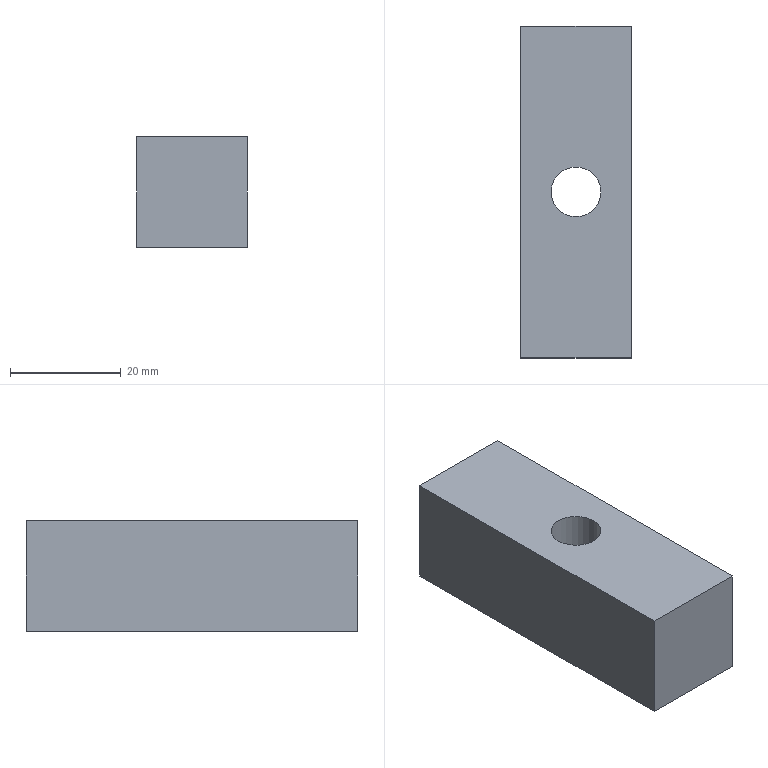Part | NX | features solid 2 | 1 solid | 9 faces | box 20 x 60 x 20 mm | volume 21824 mm3 | plane 7 | cylinder 2 | commonest cylinder face diameters 9 x1 14 x1
STEP:
#1=CARTESIAN_POINT('',(-189.,-72.007,25.));
#2=VERTEX_POINT('',#1);
#3=CARTESIAN_POINT('',(-189.,-12.007,25.));
#4=VERTEX_POINT('',#3);
#5=CARTESIAN_POINT('',(-189.,-72.007,25.));
#6=DIRECTION('',(0.,1.,0.));
#7=VECTOR('',#6,1000.);
#8=LINE('',#5,#7);
#9=EDGE_CURVE('',#2,#4,#8,.T.);
#10=ORIENTED_EDGE('',*,*,#9,.T.);
#11=CARTESIAN_POINT('',(-169.,-12.007,25.));
#12=VERTEX_POINT('',#11);
#13=CARTESIAN_POINT('',(-189.,-12.007,25.));
#14=DIRECTION('',(1.,0.,0.));
#15=VECTOR('',#14,1000.);
#16=LINE('',#13,#15);
#17=EDGE_CURVE('',#4,#12,#16,.T.);
#18=ORIENTED_EDGE('',*,*,#17,.T.);
#19=CARTESIAN_POINT('',(-169.,-72.007,25.));
#20=VERTEX_POINT('',#19);
#21=CARTESIAN_POINT('',(-169.,-12.007,25.));
#22=DIRECTION('',(0.,-1.,0.));
#23=VECTOR('',#22,1000.);
#24=LINE('',#21,#23);
#25=EDGE_CURVE('',#12,#20,#24,.T.);
#26=ORIENTED_EDGE('',*,*,#25,.T.);
#27=CARTESIAN_POINT('',(-169.,-72.007,25.));
#28=DIRECTION('',(-1.,0.,0.));
#29=VECTOR('',#28,1000.);
#30=LINE('',#27,#29);
#31=EDGE_CURVE('',#20,#2,#30,.T.);
#32=ORIENTED_EDGE('',*,*,#31,.T.);
#33=EDGE_LOOP('',(#10,#18,#26,#32));
#34=FACE_BOUND('',#33,.T.);
#35=CARTESIAN_POINT('',(-186.,-42.007,25.));
#36=VERTEX_POINT('',#35);
#37=CARTESIAN_POINT('',(-179.,-42.007,25.));
#38=DIRECTION('',(0.,0.,-1.));
#39=DIRECTION('',(-1.,0.,0.));
#40=AXIS2_PLACEMENT_3D('',#37,#38,#39);
#41=CIRCLE('',#40,7.);
#42=EDGE_CURVE('',#36,#36,#41,.F.);
#43=ORIENTED_EDGE('',*,*,#42,.T.);
#44=EDGE_LOOP('',(#43));
#45=FACE_BOUND('',#44,.T.);
#46=CARTESIAN_POINT('',(-189.,-12.007,25.));
#47=DIRECTION('',(0.,0.,-1.));
#48=DIRECTION('',(-1.,0.,0.));
#49=AXIS2_PLACEMENT_3D('',#46,#47,#48);
#50=PLANE('',#49);
#51=ADVANCED_FACE('',(#34,#45),#50,.T.);
#52=CARTESIAN_POINT('',(-183.5,-42.007,45.));
#53=VERTEX_POINT('',#52);
#54=CARTESIAN_POINT('',(-179.,-42.007,45.));
#55=DIRECTION('',(0.,0.,-1.));
#56=DIRECTION('',(-1.,0.,0.));
#57=AXIS2_PLACEMENT_3D('',#54,#55,#56);
#58=CIRCLE('',#57,4.5);
#59=EDGE_CURVE('',#53,#53,#58,.T.);
#60=ORIENTED_EDGE('',*,*,#59,.F.);
#61=EDGE_LOOP('',(#60));
#62=FACE_BOUND('',#61,.T.);
#63=CARTESIAN_POINT('',(-183.5,-42.007,35.));
#64=VERTEX_POINT('',#63);
#65=CARTESIAN_POINT('',(-179.,-42.007,35.));
#66=DIRECTION('',(0.,0.,-1.));
#67=DIRECTION('',(-1.,0.,0.));
#68=AXIS2_PLACEMENT_3D('',#65,#66,#67);
#69=CIRCLE('',#68,4.5);
#70=EDGE_CURVE('',#64,#64,#69,.T.);
#71=ORIENTED_EDGE('',*,*,#70,.T.);
#72=EDGE_LOOP('',(#71));
#73=FACE_BOUND('',#72,.T.);
#74=CARTESIAN_POINT('',(-179.,-42.007,25.));
#75=DIRECTION('',(0.,0.,1.));
#76=DIRECTION('',(1.,0.,0.));
#77=AXIS2_PLACEMENT_3D('',#74,#75,#76);
#78=CYLINDRICAL_SURFACE('',#77,4.5);
#79=ADVANCED_FACE('',(#62,#73),#78,.F.);
#80=CARTESIAN_POINT('',(-189.,-72.007,45.));
#81=VERTEX_POINT('',#80);
#82=CARTESIAN_POINT('',(-189.,-12.007,45.));
#83=VERTEX_POINT('',#82);
#84=CARTESIAN_POINT('',(-189.,-72.007,45.));
#85=DIRECTION('',(0.,1.,0.));
#86=VECTOR('',#85,1000.);
#87=LINE('',#84,#86);
#88=EDGE_CURVE('',#81,#83,#87,.T.);
#89=ORIENTED_EDGE('',*,*,#88,.F.);
#90=CARTESIAN_POINT('',(-169.,-72.007,45.));
#91=VERTEX_POINT('',#90);
#92=CARTESIAN_POINT('',(-169.,-72.007,45.));
#93=DIRECTION('',(-1.,0.,0.));
#94=VECTOR('',#93,1000.);
#95=LINE('',#92,#94);
#96=EDGE_CURVE('',#91,#81,#95,.T.);
#97=ORIENTED_EDGE('',*,*,#96,.F.);
#98=CARTESIAN_POINT('',(-169.,-12.007,45.));
#99=VERTEX_POINT('',#98);
#100=CARTESIAN_POINT('',(-169.,-12.007,45.));
#101=DIRECTION('',(0.,-1.,0.));
#102=VECTOR('',#101,1000.);
#103=LINE('',#100,#102);
#104=EDGE_CURVE('',#99,#91,#103,.T.);
#105=ORIENTED_EDGE('',*,*,#104,.F.);
#106=CARTESIAN_POINT('',(-189.,-12.007,45.));
#107=DIRECTION('',(1.,0.,0.));
#108=VECTOR('',#107,1000.);
#109=LINE('',#106,#108);
#110=EDGE_CURVE('',#83,#99,#109,.T.);
#111=ORIENTED_EDGE('',*,*,#110,.F.);
#112=EDGE_LOOP('',(#89,#97,#105,#111));
#113=FACE_BOUND('',#112,.T.);
#114=ORIENTED_EDGE('',*,*,#59,.T.);
#115=EDGE_LOOP('',(#114));
#116=FACE_BOUND('',#115,.T.);
#117=CARTESIAN_POINT('',(-189.,-12.007,45.));
#118=DIRECTION('',(0.,0.,-1.));
#119=DIRECTION('',(-1.,0.,0.));
#120=AXIS2_PLACEMENT_3D('',#117,#118,#119);
#121=PLANE('',#120);
#122=ADVANCED_FACE('',(#113,#116),#121,.F.);
#123=ORIENTED_EDGE('',*,*,#88,.T.);
#124=CARTESIAN_POINT('',(-189.,-12.007,25.));
#125=DIRECTION('',(0.,0.,1.));
#126=VECTOR('',#125,1000.);
#127=LINE('',#124,#126);
#128=EDGE_CURVE('',#4,#83,#127,.T.);
#129=ORIENTED_EDGE('',*,*,#128,.F.);
#130=ORIENTED_EDGE('',*,*,#9,.F.);
#131=CARTESIAN_POINT('',(-189.,-72.007,25.));
#132=DIRECTION('',(0.,0.,1.));
#133=VECTOR('',#132,1000.);
#134=LINE('',#131,#133);
#135=EDGE_CURVE('',#2,#81,#134,.T.);
#136=ORIENTED_EDGE('',*,*,#135,.T.);
#137=EDGE_LOOP('',(#123,#129,#130,#136));
#138=FACE_BOUND('',#137,.T.);
#139=CARTESIAN_POINT('',(-189.,-72.007,25.));
#140=DIRECTION('',(1.,0.,0.));
#141=DIRECTION('',(0.,0.,-1.));
#142=AXIS2_PLACEMENT_3D('',#139,#140,#141);
#143=PLANE('',#142);
#144=ADVANCED_FACE('',(#138),#143,.F.);
#145=ORIENTED_EDGE('',*,*,#110,.T.);
#146=CARTESIAN_POINT('',(-169.,-12.007,25.));
#147=DIRECTION('',(0.,0.,1.));
#148=VECTOR('',#147,1000.);
#149=LINE('',#146,#148);
#150=EDGE_CURVE('',#12,#99,#149,.T.);
#151=ORIENTED_EDGE('',*,*,#150,.F.);
#152=ORIENTED_EDGE('',*,*,#17,.F.);
#153=ORIENTED_EDGE('',*,*,#128,.T.);
#154=EDGE_LOOP('',(#145,#151,#152,#153));
#155=FACE_BOUND('',#154,.T.);
#156=CARTESIAN_POINT('',(-189.,-12.007,25.));
#157=DIRECTION('',(0.,-1.,0.));
#158=DIRECTION('',(0.,0.,-1.));
#159=AXIS2_PLACEMENT_3D('',#156,#157,#158);
#160=PLANE('',#159);
#161=ADVANCED_FACE('',(#155),#160,.F.);
#162=ORIENTED_EDGE('',*,*,#104,.T.);
#163=CARTESIAN_POINT('',(-169.,-72.007,25.));
#164=DIRECTION('',(0.,0.,1.));
#165=VECTOR('',#164,1000.);
#166=LINE('',#163,#165);
#167=EDGE_CURVE('',#20,#91,#166,.T.);
#168=ORIENTED_EDGE('',*,*,#167,.F.);
#169=ORIENTED_EDGE('',*,*,#25,.F.);
#170=ORIENTED_EDGE('',*,*,#150,.T.);
#171=EDGE_LOOP('',(#162,#168,#169,#170));
#172=FACE_BOUND('',#171,.T.);
#173=CARTESIAN_POINT('',(-169.,-12.007,25.));
#174=DIRECTION('',(-1.,0.,0.));
#175=DIRECTION('',(0.,0.,1.));
#176=AXIS2_PLACEMENT_3D('',#173,#174,#175);
#177=PLANE('',#176);
#178=ADVANCED_FACE('',(#172),#177,.F.);
#179=ORIENTED_EDGE('',*,*,#96,.T.);
#180=ORIENTED_EDGE('',*,*,#135,.F.);
#181=ORIENTED_EDGE('',*,*,#31,.F.);
#182=ORIENTED_EDGE('',*,*,#167,.T.);
#183=EDGE_LOOP('',(#179,#180,#181,#182));
#184=FACE_BOUND('',#183,.T.);
#185=CARTESIAN_POINT('',(-169.,-72.007,25.));
#186=DIRECTION('',(0.,1.,0.));
#187=DIRECTION('',(0.,0.,1.));
#188=AXIS2_PLACEMENT_3D('',#185,#186,#187);
#189=PLANE('',#188);
#190=ADVANCED_FACE('',(#184),#189,.F.);
#191=ORIENTED_EDGE('',*,*,#42,.F.);
#192=EDGE_LOOP('',(#191));
#193=FACE_BOUND('',#192,.T.);
#194=CARTESIAN_POINT('',(-186.,-42.007,35.));
#195=VERTEX_POINT('',#194);
#196=CARTESIAN_POINT('',(-179.,-42.007,35.));
#197=DIRECTION('',(0.,0.,-1.));
#198=DIRECTION('',(-1.,0.,0.));
#199=AXIS2_PLACEMENT_3D('',#196,#197,#198);
#200=CIRCLE('',#199,7.);
#201=EDGE_CURVE('',#195,#195,#200,.T.);
#202=ORIENTED_EDGE('',*,*,#201,.F.);
#203=EDGE_LOOP('',(#202));
#204=FACE_BOUND('',#203,.T.);
#205=CARTESIAN_POINT('',(-179.,-42.007,15.));
#206=DIRECTION('',(0.,0.,1.));
#207=DIRECTION('',(1.,0.,0.));
#208=AXIS2_PLACEMENT_3D('',#205,#206,#207);
#209=CYLINDRICAL_SURFACE('',#208,7.);
#210=ADVANCED_FACE('',(#193,#204),#209,.F.);
#211=ORIENTED_EDGE('',*,*,#70,.F.);
#212=EDGE_LOOP('',(#211));
#213=FACE_BOUND('',#212,.T.);
#214=ORIENTED_EDGE('',*,*,#201,.T.);
#215=EDGE_LOOP('',(#214));
#216=FACE_BOUND('',#215,.T.);
#217=CARTESIAN_POINT('',(-179.,-42.007,35.));
#218=DIRECTION('',(0.,0.,-1.));
#219=DIRECTION('',(-1.,0.,0.));
#220=AXIS2_PLACEMENT_3D('',#217,#218,#219);
#221=PLANE('',#220);
#222=ADVANCED_FACE('',(#213,#216),#221,.T.);
#223=CLOSED_SHELL('',(#51,#79,#122,#144,#161,#178,#190,#210,#222));
#224=MANIFOLD_SOLID_BREP('',#223);
#225=(LENGTH_UNIT()NAMED_UNIT(*)SI_UNIT(.MILLI.,.METRE.));
#226=UNCERTAINTY_MEASURE_WITH_UNIT(LENGTH_MEASURE(0.00001),#225,'','');
#227=(NAMED_UNIT(*)PLANE_ANGLE_UNIT()SI_UNIT($,.RADIAN.));
#228=(NAMED_UNIT(*)SI_UNIT($,.STERADIAN.)SOLID_ANGLE_UNIT());
#229=(GEOMETRIC_REPRESENTATION_CONTEXT(3)GLOBAL_UNCERTAINTY_ASSIGNED_CONTEXT((#226))GLOBAL_UNIT_ASSIGNED_CONTEXT((#225,#227,#228))REPRESENTATION_CONTEXT('',''));
#230=ADVANCED_BREP_SHAPE_REPRESENTATION('',(#224),#229);